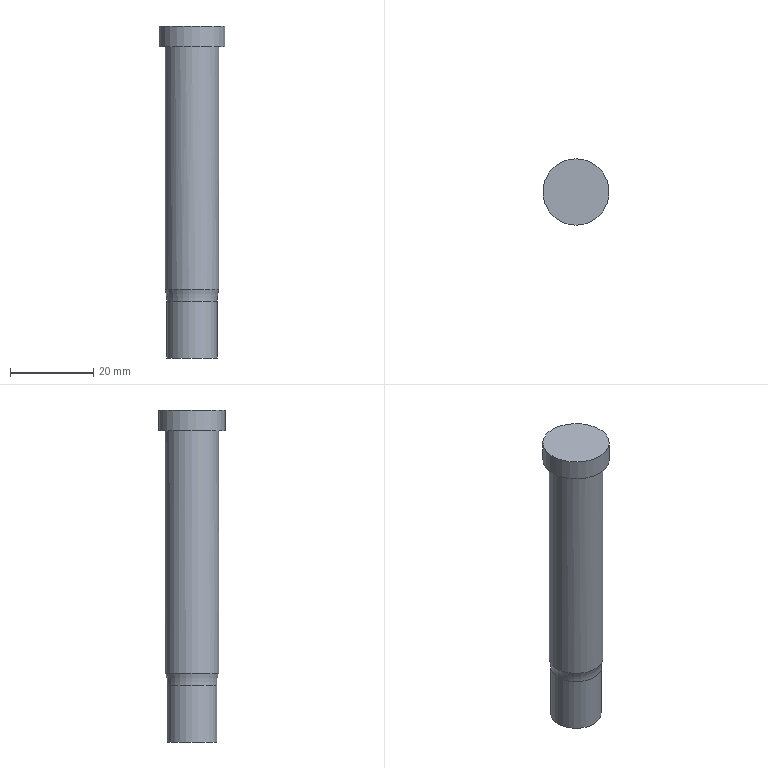Part | NX | features MAIN_BODY 2 | 1 solid | 7 faces | box 16 x 16 x 80 mm | volume 10683 mm3 | cylinder 3 | plane 3 | torus 1 | commonest cylinder face diameters 12.1 x1 13 x1 16 x1
STEP:
#1=CARTESIAN_POINT('',(1484.996,634.778,-4.466));
#2=VERTEX_POINT('',#1);
#3=CARTESIAN_POINT('',(1491.496,634.778,-4.466));
#4=DIRECTION('',(0.,0.,-1.));
#5=DIRECTION('',(-1.,0.,0.));
#6=AXIS2_PLACEMENT_3D('',#3,#4,#5);
#7=CIRCLE('',#6,6.5);
#8=EDGE_CURVE('',#2,#2,#7,.T.);
#9=ORIENTED_EDGE('',*,*,#8,.F.);
#10=EDGE_LOOP('',(#9));
#11=FACE_BOUND('',#10,.T.);
#12=CARTESIAN_POINT('',(1491.496,628.278,54.));
#13=VERTEX_POINT('',#12);
#14=CARTESIAN_POINT('',(1491.496,634.778,54.));
#15=DIRECTION('',(0.,0.,-1.));
#16=DIRECTION('',(0.,-1.,0.));
#17=AXIS2_PLACEMENT_3D('',#14,#15,#16);
#18=CIRCLE('',#17,6.5);
#19=EDGE_CURVE('',#13,#13,#18,.T.);
#20=ORIENTED_EDGE('',*,*,#19,.T.);
#21=EDGE_LOOP('',(#20));
#22=FACE_BOUND('',#21,.T.);
#23=CARTESIAN_POINT('',(1491.496,634.778,59.));
#24=DIRECTION('',(0.,0.,-1.));
#25=DIRECTION('',(0.,1.,0.));
#26=AXIS2_PLACEMENT_3D('',#23,#24,#25);
#27=CYLINDRICAL_SURFACE('',#26,6.5);
#28=ADVANCED_FACE('',(#11,#22),#27,.T.);
#29=CARTESIAN_POINT('',(1491.496,626.778,54.));
#30=VERTEX_POINT('',#29);
#31=CARTESIAN_POINT('',(1491.496,634.778,54.));
#32=DIRECTION('',(0.,0.,-1.));
#33=DIRECTION('',(0.,-1.,0.));
#34=AXIS2_PLACEMENT_3D('',#31,#32,#33);
#35=CIRCLE('',#34,8.);
#36=EDGE_CURVE('',#30,#30,#35,.T.);
#37=ORIENTED_EDGE('',*,*,#36,.T.);
#38=EDGE_LOOP('',(#37));
#39=FACE_BOUND('',#38,.T.);
#40=ORIENTED_EDGE('',*,*,#19,.F.);
#41=EDGE_LOOP('',(#40));
#42=FACE_BOUND('',#41,.T.);
#43=CARTESIAN_POINT('',(1491.496,634.778,54.));
#44=DIRECTION('',(0.,0.,1.));
#45=DIRECTION('',(0.,-1.,0.));
#46=AXIS2_PLACEMENT_3D('',#43,#44,#45);
#47=PLANE('',#46);
#48=ADVANCED_FACE('',(#39,#42),#47,.F.);
#49=ORIENTED_EDGE('',*,*,#36,.F.);
#50=EDGE_LOOP('',(#49));
#51=FACE_BOUND('',#50,.T.);
#52=CARTESIAN_POINT('',(1491.496,626.778,59.));
#53=VERTEX_POINT('',#52);
#54=CARTESIAN_POINT('',(1491.496,634.778,59.));
#55=DIRECTION('',(0.,0.,-1.));
#56=DIRECTION('',(0.,-1.,0.));
#57=AXIS2_PLACEMENT_3D('',#54,#55,#56);
#58=CIRCLE('',#57,8.);
#59=EDGE_CURVE('',#53,#53,#58,.T.);
#60=ORIENTED_EDGE('',*,*,#59,.T.);
#61=EDGE_LOOP('',(#60));
#62=FACE_BOUND('',#61,.T.);
#63=CARTESIAN_POINT('',(1491.496,634.778,55.));
#64=DIRECTION('',(0.,0.,1.));
#65=DIRECTION('',(0.,-1.,0.));
#66=AXIS2_PLACEMENT_3D('',#63,#64,#65);
#67=CYLINDRICAL_SURFACE('',#66,8.);
#68=ADVANCED_FACE('',(#51,#62),#67,.T.);
#69=ORIENTED_EDGE('',*,*,#59,.F.);
#70=EDGE_LOOP('',(#69));
#71=FACE_BOUND('',#70,.T.);
#72=CARTESIAN_POINT('',(1491.496,634.778,59.));
#73=DIRECTION('',(0.,0.,1.));
#74=DIRECTION('',(0.,-1.,0.));
#75=AXIS2_PLACEMENT_3D('',#72,#73,#74);
#76=PLANE('',#75);
#77=ADVANCED_FACE('',(#71),#76,.T.);
#78=CARTESIAN_POINT('',(1497.546,634.778,-7.268));
#79=VERTEX_POINT('',#78);
#80=CARTESIAN_POINT('',(1491.496,634.778,-7.268));
#81=DIRECTION('',(0.,0.,1.));
#82=DIRECTION('',(1.,0.,0.));
#83=AXIS2_PLACEMENT_3D('',#80,#81,#82);
#84=CIRCLE('',#83,6.05);
#85=EDGE_CURVE('',#79,#79,#84,.T.);
#86=ORIENTED_EDGE('',*,*,#85,.F.);
#87=EDGE_LOOP('',(#86));
#88=FACE_BOUND('',#87,.T.);
#89=CARTESIAN_POINT('',(1497.546,634.778,-21.));
#90=VERTEX_POINT('',#89);
#91=CARTESIAN_POINT('',(1491.496,634.778,-21.));
#92=DIRECTION('',(0.,0.,1.));
#93=DIRECTION('',(1.,0.,0.));
#94=AXIS2_PLACEMENT_3D('',#91,#92,#93);
#95=CIRCLE('',#94,6.05);
#96=EDGE_CURVE('',#90,#90,#95,.F.);
#97=ORIENTED_EDGE('',*,*,#96,.F.);
#98=EDGE_LOOP('',(#97));
#99=FACE_BOUND('',#98,.T.);
#100=CARTESIAN_POINT('',(1491.496,634.778,-21.));
#101=DIRECTION('',(0.,0.,1.));
#102=DIRECTION('',(0.,-1.,0.));
#103=AXIS2_PLACEMENT_3D('',#100,#101,#102);
#104=CYLINDRICAL_SURFACE('',#103,6.05);
#105=ADVANCED_FACE('',(#88,#99),#104,.T.);
#106=ORIENTED_EDGE('',*,*,#96,.T.);
#107=EDGE_LOOP('',(#106));
#108=FACE_BOUND('',#107,.T.);
#109=CARTESIAN_POINT('',(1491.496,634.778,-21.));
#110=DIRECTION('',(0.,0.,1.));
#111=DIRECTION('',(0.,-1.,0.));
#112=AXIS2_PLACEMENT_3D('',#109,#110,#111);
#113=PLANE('',#112);
#114=ADVANCED_FACE('',(#108),#113,.F.);
#115=ORIENTED_EDGE('',*,*,#85,.T.);
#116=EDGE_LOOP('',(#115));
#117=FACE_BOUND('',#116,.T.);
#118=ORIENTED_EDGE('',*,*,#8,.T.);
#119=EDGE_LOOP('',(#118));
#120=FACE_BOUND('',#119,.T.);
#121=CARTESIAN_POINT('',(1491.496,634.778,-7.268));
#122=DIRECTION('',(0.,0.,1.));
#123=DIRECTION('',(0.,-1.,0.));
#124=AXIS2_PLACEMENT_3D('',#121,#122,#123);
#125=TOROIDAL_SURFACE('',#124,15.,8.95);
#126=ADVANCED_FACE('',(#117,#120),#125,.F.);
#127=CLOSED_SHELL('',(#28,#48,#68,#77,#105,#114,#126));
#128=MANIFOLD_SOLID_BREP('',#127);
#129=(LENGTH_UNIT()NAMED_UNIT(*)SI_UNIT(.MILLI.,.METRE.));
#130=UNCERTAINTY_MEASURE_WITH_UNIT(LENGTH_MEASURE(0.00001),#129,'','');
#131=(NAMED_UNIT(*)PLANE_ANGLE_UNIT()SI_UNIT($,.RADIAN.));
#132=(NAMED_UNIT(*)SI_UNIT($,.STERADIAN.)SOLID_ANGLE_UNIT());
#133=(GEOMETRIC_REPRESENTATION_CONTEXT(3)GLOBAL_UNCERTAINTY_ASSIGNED_CONTEXT((#130))GLOBAL_UNIT_ASSIGNED_CONTEXT((#129,#131,#132))REPRESENTATION_CONTEXT('',''));
#134=ADVANCED_BREP_SHAPE_REPRESENTATION('',(#128),#133);